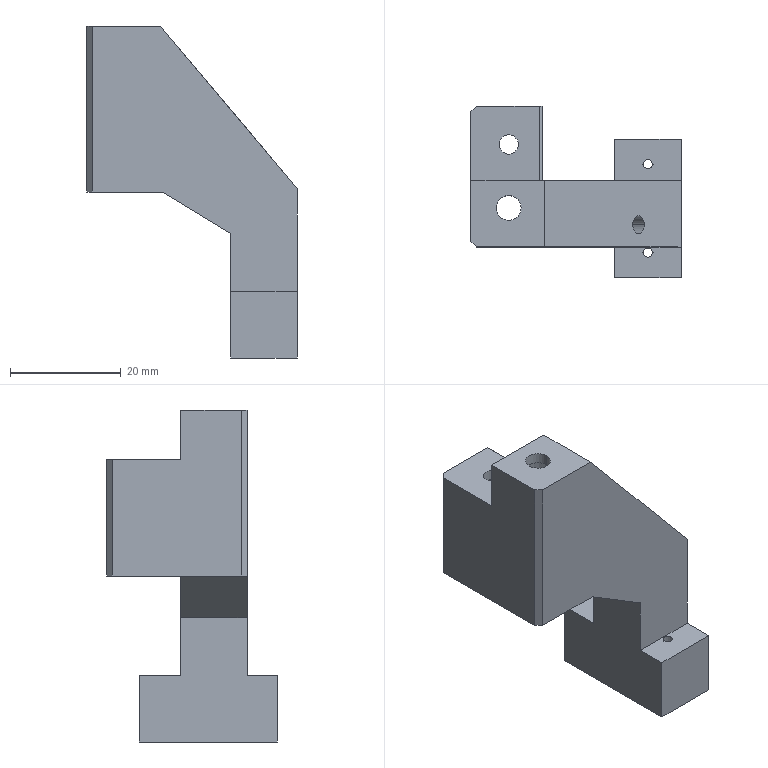Part | SolidWorks | features ICE 14, HoleWzd 5, Chamfer 2, Extrusion 1 | 1 solid | 62 faces | box 38 x 30.9 x 60 mm | volume 16944 mm3 | cylinder 24 | plane 22 | cone 16 | commonest cylinder face diameters 3.3 x8 1.6 x4 3 x4 3.5 x2 4.5 x2 7 x2